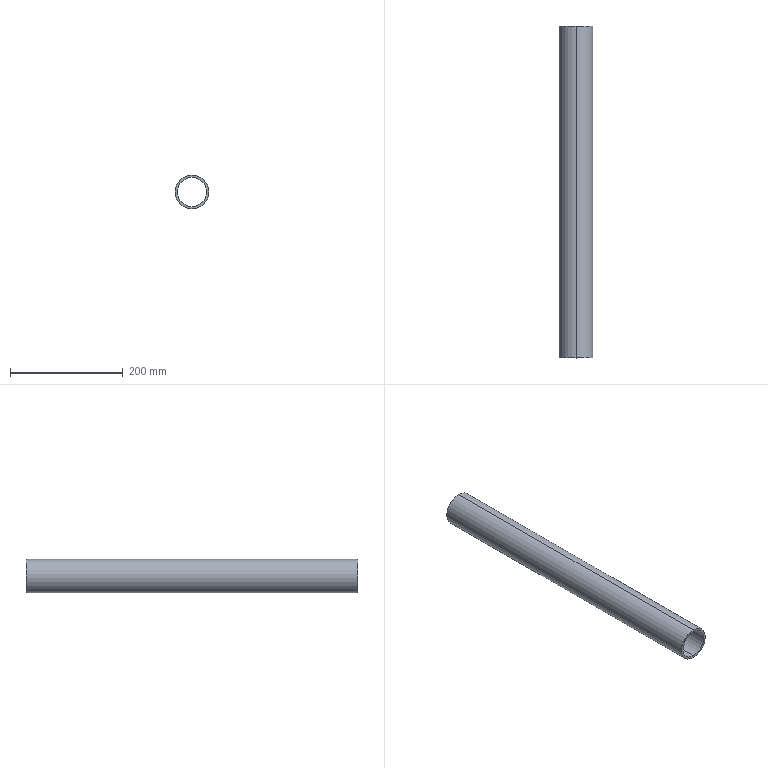Part | SolidWorks | features WeldMemberFeat 1, WeldmentFeature 1 | 1 solid | 6 faces | box 60 x 590 x 60 mm | volume 415193 mm3 | cylinder 4 | plane 2 | commonest cylinder face diameters 52 x2 60 x2
STEP:
#1=CARTESIAN_POINT('',(0.,590.,30.));
#2=VERTEX_POINT('',#1);
#3=CARTESIAN_POINT('',(0.,590.,-30.));
#4=VERTEX_POINT('',#3);
#5=CARTESIAN_POINT('',(0.,590.,0.));
#6=DIRECTION('',(0.,1.,0.));
#7=DIRECTION('',(0.,0.,1.));
#8=AXIS2_PLACEMENT_3D('',#5,#6,#7);
#9=CIRCLE('',#8,30.);
#10=EDGE_CURVE('',#2,#4,#9,.T.);
#11=ORIENTED_EDGE('',*,*,#10,.F.);
#12=CARTESIAN_POINT('',(0.,0.,30.));
#13=VERTEX_POINT('',#12);
#14=CARTESIAN_POINT('',(0.,590.,30.));
#15=DIRECTION('',(0.,-1.,0.));
#16=VECTOR('',#15,1000.);
#17=LINE('',#14,#16);
#18=EDGE_CURVE('',#2,#13,#17,.T.);
#19=ORIENTED_EDGE('',*,*,#18,.T.);
#20=CARTESIAN_POINT('',(0.,0.,-30.));
#21=VERTEX_POINT('',#20);
#22=CARTESIAN_POINT('',(0.,0.,0.));
#23=DIRECTION('',(0.,1.,0.));
#24=DIRECTION('',(0.,0.,1.));
#25=AXIS2_PLACEMENT_3D('',#22,#23,#24);
#26=CIRCLE('',#25,30.);
#27=EDGE_CURVE('',#13,#21,#26,.T.);
#28=ORIENTED_EDGE('',*,*,#27,.T.);
#29=CARTESIAN_POINT('',(0.,590.,-30.));
#30=DIRECTION('',(0.,-1.,0.));
#31=VECTOR('',#30,1000.);
#32=LINE('',#29,#31);
#33=EDGE_CURVE('',#4,#21,#32,.T.);
#34=ORIENTED_EDGE('',*,*,#33,.F.);
#35=EDGE_LOOP('',(#11,#19,#28,#34));
#36=FACE_OUTER_BOUND('',#35,.T.);
#37=CARTESIAN_POINT('',(0.,590.,0.));
#38=DIRECTION('',(0.,-1.,0.));
#39=DIRECTION('',(0.,0.,-1.));
#40=AXIS2_PLACEMENT_3D('',#37,#38,#39);
#41=CYLINDRICAL_SURFACE('',#40,30.);
#42=ADVANCED_FACE('',(#36),#41,.T.);
#43=CARTESIAN_POINT('',(0.,590.,-26.));
#44=VERTEX_POINT('',#43);
#45=CARTESIAN_POINT('',(0.,590.,26.));
#46=VERTEX_POINT('',#45);
#47=CARTESIAN_POINT('',(0.,590.,0.));
#48=DIRECTION('',(0.,1.,0.));
#49=DIRECTION('',(0.,0.,1.));
#50=AXIS2_PLACEMENT_3D('',#47,#48,#49);
#51=CIRCLE('',#50,26.);
#52=EDGE_CURVE('',#44,#46,#51,.T.);
#53=ORIENTED_EDGE('',*,*,#52,.T.);
#54=CARTESIAN_POINT('',(0.,0.,26.));
#55=VERTEX_POINT('',#54);
#56=CARTESIAN_POINT('',(0.,590.,26.));
#57=DIRECTION('',(0.,-1.,0.));
#58=VECTOR('',#57,1000.);
#59=LINE('',#56,#58);
#60=EDGE_CURVE('',#46,#55,#59,.T.);
#61=ORIENTED_EDGE('',*,*,#60,.T.);
#62=CARTESIAN_POINT('',(0.,0.,-26.));
#63=VERTEX_POINT('',#62);
#64=CARTESIAN_POINT('',(0.,0.,0.));
#65=DIRECTION('',(0.,1.,0.));
#66=DIRECTION('',(0.,0.,1.));
#67=AXIS2_PLACEMENT_3D('',#64,#65,#66);
#68=CIRCLE('',#67,26.);
#69=EDGE_CURVE('',#63,#55,#68,.T.);
#70=ORIENTED_EDGE('',*,*,#69,.F.);
#71=CARTESIAN_POINT('',(0.,590.,-26.));
#72=DIRECTION('',(0.,-1.,0.));
#73=VECTOR('',#72,1000.);
#74=LINE('',#71,#73);
#75=EDGE_CURVE('',#44,#63,#74,.T.);
#76=ORIENTED_EDGE('',*,*,#75,.F.);
#77=EDGE_LOOP('',(#53,#61,#70,#76));
#78=FACE_OUTER_BOUND('',#77,.T.);
#79=CARTESIAN_POINT('',(0.,590.,0.));
#80=DIRECTION('',(0.,-1.,0.));
#81=DIRECTION('',(0.,0.,-1.));
#82=AXIS2_PLACEMENT_3D('',#79,#80,#81);
#83=CYLINDRICAL_SURFACE('',#82,26.);
#84=ADVANCED_FACE('',(#78),#83,.F.);
#85=ORIENTED_EDGE('',*,*,#60,.F.);
#86=CARTESIAN_POINT('',(0.,590.,0.));
#87=DIRECTION('',(0.,1.,0.));
#88=DIRECTION('',(0.,0.,1.));
#89=AXIS2_PLACEMENT_3D('',#86,#87,#88);
#90=CIRCLE('',#89,26.);
#91=EDGE_CURVE('',#46,#44,#90,.T.);
#92=ORIENTED_EDGE('',*,*,#91,.T.);
#93=ORIENTED_EDGE('',*,*,#75,.T.);
#94=CARTESIAN_POINT('',(0.,0.,0.));
#95=DIRECTION('',(0.,1.,0.));
#96=DIRECTION('',(0.,0.,1.));
#97=AXIS2_PLACEMENT_3D('',#94,#95,#96);
#98=CIRCLE('',#97,26.);
#99=EDGE_CURVE('',#55,#63,#98,.T.);
#100=ORIENTED_EDGE('',*,*,#99,.F.);
#101=EDGE_LOOP('',(#85,#92,#93,#100));
#102=FACE_OUTER_BOUND('',#101,.T.);
#103=CARTESIAN_POINT('',(0.,590.,0.));
#104=DIRECTION('',(0.,-1.,0.));
#105=DIRECTION('',(0.,0.,-1.));
#106=AXIS2_PLACEMENT_3D('',#103,#104,#105);
#107=CYLINDRICAL_SURFACE('',#106,26.);
#108=ADVANCED_FACE('',(#102),#107,.F.);
#109=ORIENTED_EDGE('',*,*,#18,.F.);
#110=CARTESIAN_POINT('',(0.,590.,0.));
#111=DIRECTION('',(0.,1.,0.));
#112=DIRECTION('',(0.,0.,1.));
#113=AXIS2_PLACEMENT_3D('',#110,#111,#112);
#114=CIRCLE('',#113,30.);
#115=EDGE_CURVE('',#4,#2,#114,.T.);
#116=ORIENTED_EDGE('',*,*,#115,.F.);
#117=ORIENTED_EDGE('',*,*,#33,.T.);
#118=CARTESIAN_POINT('',(0.,0.,0.));
#119=DIRECTION('',(0.,1.,0.));
#120=DIRECTION('',(0.,0.,1.));
#121=AXIS2_PLACEMENT_3D('',#118,#119,#120);
#122=CIRCLE('',#121,30.);
#123=EDGE_CURVE('',#21,#13,#122,.T.);
#124=ORIENTED_EDGE('',*,*,#123,.T.);
#125=EDGE_LOOP('',(#109,#116,#117,#124));
#126=FACE_OUTER_BOUND('',#125,.T.);
#127=CARTESIAN_POINT('',(0.,590.,0.));
#128=DIRECTION('',(0.,-1.,0.));
#129=DIRECTION('',(0.,0.,-1.));
#130=AXIS2_PLACEMENT_3D('',#127,#128,#129);
#131=CYLINDRICAL_SURFACE('',#130,30.);
#132=ADVANCED_FACE('',(#126),#131,.T.);
#133=ORIENTED_EDGE('',*,*,#52,.F.);
#134=ORIENTED_EDGE('',*,*,#91,.F.);
#135=EDGE_LOOP('',(#133,#134));
#136=FACE_BOUND('',#135,.T.);
#137=ORIENTED_EDGE('',*,*,#115,.T.);
#138=ORIENTED_EDGE('',*,*,#10,.T.);
#139=EDGE_LOOP('',(#137,#138));
#140=FACE_OUTER_BOUND('',#139,.T.);
#141=CARTESIAN_POINT('',(0.,590.,0.));
#142=DIRECTION('',(0.,1.,0.));
#143=DIRECTION('',(0.,0.,1.));
#144=AXIS2_PLACEMENT_3D('',#141,#142,#143);
#145=PLANE('',#144);
#146=ADVANCED_FACE('',(#136,#140),#145,.T.);
#147=ORIENTED_EDGE('',*,*,#69,.T.);
#148=ORIENTED_EDGE('',*,*,#99,.T.);
#149=EDGE_LOOP('',(#147,#148));
#150=FACE_BOUND('',#149,.T.);
#151=ORIENTED_EDGE('',*,*,#123,.F.);
#152=ORIENTED_EDGE('',*,*,#27,.F.);
#153=EDGE_LOOP('',(#151,#152));
#154=FACE_OUTER_BOUND('',#153,.T.);
#155=CARTESIAN_POINT('',(0.,0.,0.));
#156=DIRECTION('',(0.,1.,0.));
#157=DIRECTION('',(0.,0.,1.));
#158=AXIS2_PLACEMENT_3D('',#155,#156,#157);
#159=PLANE('',#158);
#160=ADVANCED_FACE('',(#150,#154),#159,.F.);
#161=CLOSED_SHELL('',(#42,#84,#108,#132,#146,#160));
#162=MANIFOLD_SOLID_BREP('',#161);
#163=CARTESIAN_POINT('',(0.,0.,0.));
#164=DIRECTION('',(0.,0.,1.));
#165=DIRECTION('',(1.,0.,0.));
#166=AXIS2_PLACEMENT_3D('',#163,#164,#165);
#167=(LENGTH_UNIT()NAMED_UNIT(*)SI_UNIT(.MILLI.,.METRE.));
#168=UNCERTAINTY_MEASURE_WITH_UNIT(LENGTH_MEASURE(0.00001),#167,'','');
#169=(NAMED_UNIT(*)PLANE_ANGLE_UNIT()SI_UNIT($,.RADIAN.));
#170=(NAMED_UNIT(*)SI_UNIT($,.STERADIAN.)SOLID_ANGLE_UNIT());
#171=(GEOMETRIC_REPRESENTATION_CONTEXT(3)GLOBAL_UNCERTAINTY_ASSIGNED_CONTEXT((#168))GLOBAL_UNIT_ASSIGNED_CONTEXT((#167,#169,#170))REPRESENTATION_CONTEXT('',''));
#172=ADVANCED_BREP_SHAPE_REPRESENTATION('',(#162,#166),#171);